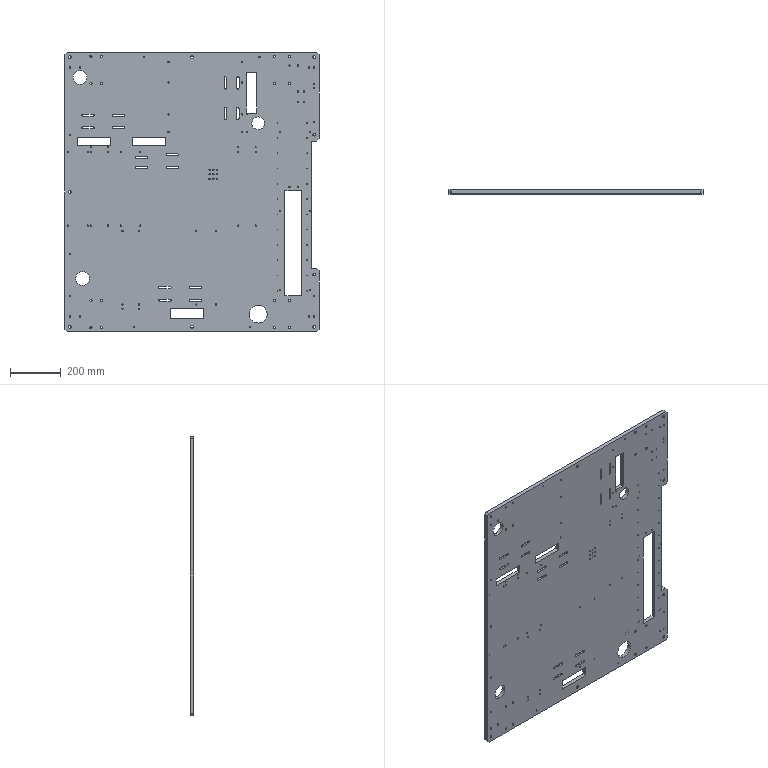Part | STEP file | 1 solid | 651 faces | box 1000 x 15 x 1100 mm | volume 15184573 mm3 | cylinder 464 | plane 165 | cone 22 | commonest cylinder face diameters 5 x120 6 x88 8.5 x68 2.5 x48 16 x44 10 x18